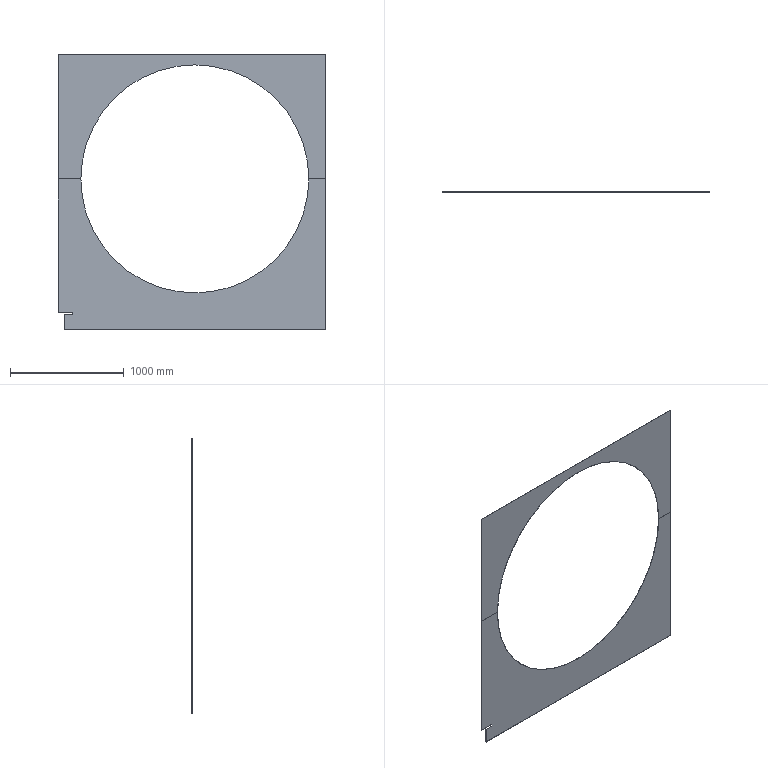Part | STEP file | Bracket花纹Plate 6 | 2 solids | 22 faces | box 2350 x 3 x 2420 mm | volume 7605664 mm3 | plane 18 | cylinder 4 | commonest cylinder face diameters 2000 x3 6 x1